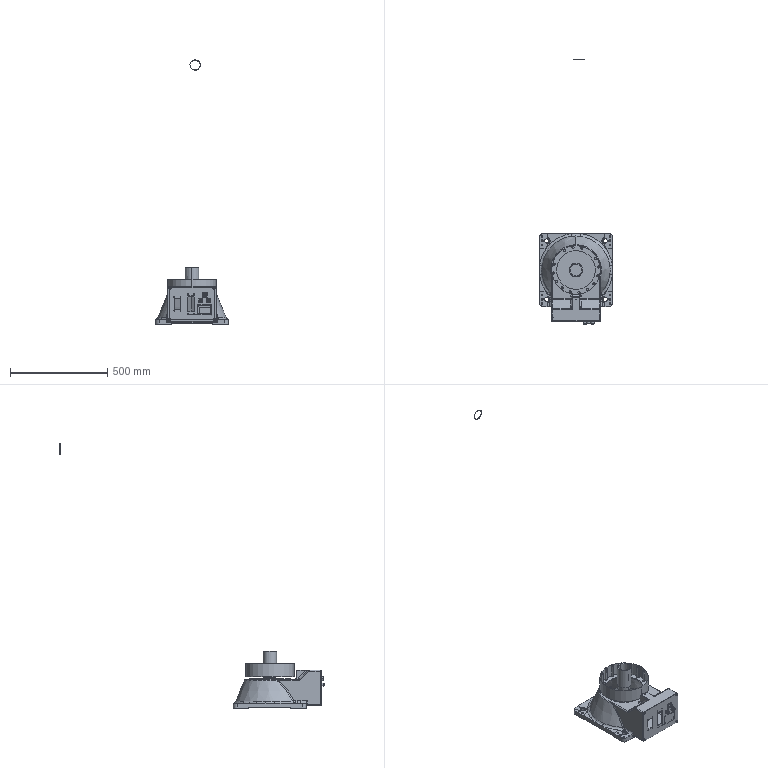Part | NX | features BREP 16 | 1 solid | 334 faces | box 375 x 1359 x 1358 mm | volume 6945201 mm3 | cylinder 153 | plane 101 | cone 31 | torus 25 | spline 22 | sphere 2 | commonest cylinder face diameters 10 x23 8.5 x16 11 x16 20 x11 4 x9 22 x8